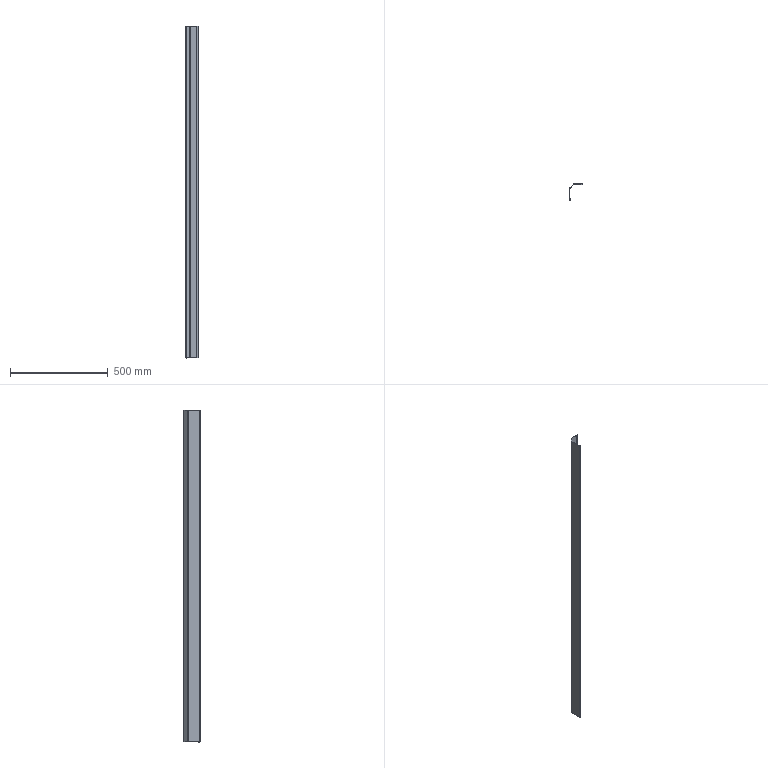Part | STEP file | 51E-01209JG10 | 1 solid | 53 faces | box 65 x 82.9 x 1700 mm | volume 350793 mm3 | cylinder 30 | plane 23 | commonest cylinder face diameters 1 x9 1.8 x6 0.9 x4 0.4 x3 0.6 x2 3 x2